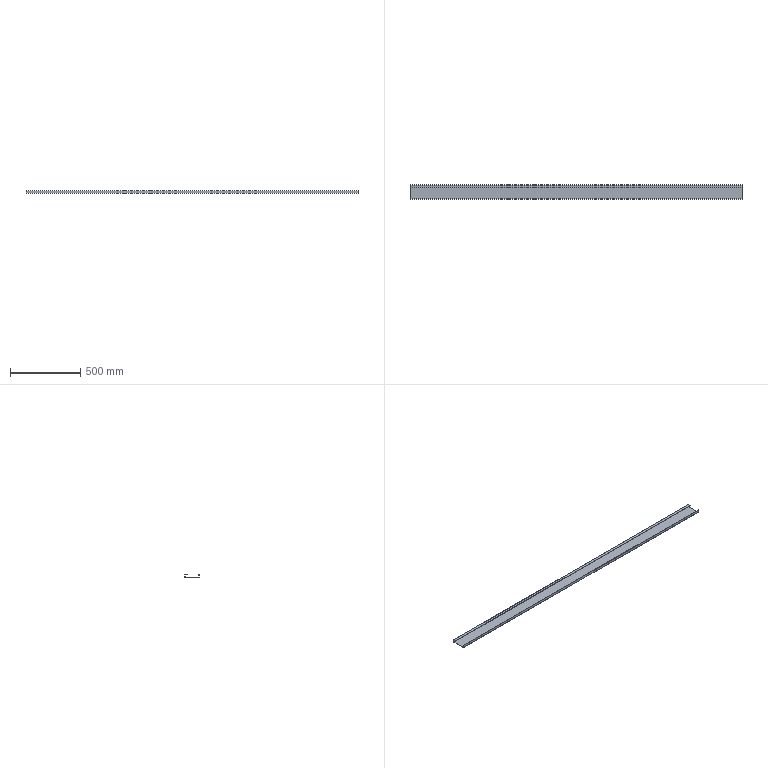Part | STEP file | 粉仓踢脚Plate 9 | 1 solid | 18 faces | box 2365 x 100 x 20 mm | volume 543643 mm3 | plane 12 | cylinder 6 | commonest cylinder face diameters 2 x3 5 x3
STEP:
#1=CARTESIAN_POINT('',(0.,0.,0.));
#2=DIRECTION('',(0.,0.,1.));
#3=DIRECTION('',(1.,0.,0.));
#4=AXIS2_PLACEMENT_3D('',#1,#2,#3);
#5=CARTESIAN_POINT('',(-1182.5,1.5,2.5));
#6=VERTEX_POINT('',#5);
#7=CARTESIAN_POINT('',(-1182.5,1.5,20.));
#8=VERTEX_POINT('',#7);
#9=CARTESIAN_POINT('',(-1182.5,1.5,2.5));
#10=DIRECTION('',(0.,0.,1.));
#11=VECTOR('',#10,1.);
#12=LINE('',#9,#11);
#13=CARTESIAN_POINT('',(1182.5,1.5,2.5));
#14=DIRECTION('',(0.,-1.,0.));
#15=DIRECTION('',(0.,0.,-1.));
#16=AXIS2_PLACEMENT_3D('',#13,#14,#15);
#17=PLANE('',#16);
#18=CARTESIAN_POINT('',(0.,-2365.));
#19=DIRECTION('',(-1.,0.));
#20=VECTOR('',#19,1.);
#21=LINE('',#18,#20);
#22=(GEOMETRIC_REPRESENTATION_CONTEXT(2)PARAMETRIC_REPRESENTATION_CONTEXT()REPRESENTATION_CONTEXT('',''));
#23=DEFINITIONAL_REPRESENTATION('',(#21),#22);
#24=PCURVE('',#17,#23);
#25=CARTESIAN_POINT('',(-1182.5,2.5,2.5));
#26=DIRECTION('',(-1.,0.,0.));
#27=DIRECTION('',(0.,0.,1.));
#28=AXIS2_PLACEMENT_3D('',#25,#26,#27);
#29=PLANE('',#28);
#30=CARTESIAN_POINT('',(0.,-1.));
#31=DIRECTION('',(1.,0.));
#32=VECTOR('',#31,1.);
#33=LINE('',#30,#32);
#34=(GEOMETRIC_REPRESENTATION_CONTEXT(2)PARAMETRIC_REPRESENTATION_CONTEXT()REPRESENTATION_CONTEXT('',''));
#35=DEFINITIONAL_REPRESENTATION('',(#33),#34);
#36=PCURVE('',#29,#35);
#37=SURFACE_CURVE('',#12,(#24,#36),.PCURVE_S1.);
#38=EDGE_CURVE('',#6,#8,#37,.T.);
#39=ORIENTED_EDGE('',*,*,#38,.T.);
#40=CARTESIAN_POINT('',(1182.5,1.5,20.));
#41=VERTEX_POINT('',#40);
#42=CARTESIAN_POINT('',(1182.5,1.5,20.));
#43=DIRECTION('',(-1.,0.,0.));
#44=VECTOR('',#43,1.);
#45=LINE('',#42,#44);
#46=CARTESIAN_POINT('',(-17.5,0.));
#47=DIRECTION('',(0.,-1.));
#48=VECTOR('',#47,1.);
#49=LINE('',#46,#48);
#50=(GEOMETRIC_REPRESENTATION_CONTEXT(2)PARAMETRIC_REPRESENTATION_CONTEXT()REPRESENTATION_CONTEXT('',''));
#51=DEFINITIONAL_REPRESENTATION('',(#49),#50);
#52=PCURVE('',#17,#51);
#53=CARTESIAN_POINT('',(1182.5,0.,20.));
#54=DIRECTION('',(0.,0.,1.));
#55=DIRECTION('',(1.,0.,0.));
#56=AXIS2_PLACEMENT_3D('',#53,#54,#55);
#57=PLANE('',#56);
#58=CARTESIAN_POINT('',(0.,1.5));
#59=DIRECTION('',(-1.,0.));
#60=VECTOR('',#59,1.);
#61=LINE('',#58,#60);
#62=(GEOMETRIC_REPRESENTATION_CONTEXT(2)PARAMETRIC_REPRESENTATION_CONTEXT()REPRESENTATION_CONTEXT('',''));
#63=DEFINITIONAL_REPRESENTATION('',(#61),#62);
#64=PCURVE('',#57,#63);
#65=SURFACE_CURVE('',#45,(#52,#64),.PCURVE_S1.);
#66=EDGE_CURVE('',#41,#8,#65,.T.);
#67=ORIENTED_EDGE('',*,*,#66,.F.);
#68=CARTESIAN_POINT('',(1182.5,1.5,2.5));
#69=VERTEX_POINT('',#68);
#70=CARTESIAN_POINT('',(1182.5,1.5,2.5));
#71=DIRECTION('',(0.,0.,1.));
#72=VECTOR('',#71,1.);
#73=LINE('',#70,#72);
#74=CARTESIAN_POINT('',(0.,0.));
#75=DIRECTION('',(-1.,0.));
#76=VECTOR('',#75,1.);
#77=LINE('',#74,#76);
#78=(GEOMETRIC_REPRESENTATION_CONTEXT(2)PARAMETRIC_REPRESENTATION_CONTEXT()REPRESENTATION_CONTEXT('',''));
#79=DEFINITIONAL_REPRESENTATION('',(#77),#78);
#80=PCURVE('',#17,#79);
#81=CARTESIAN_POINT('',(1182.5,2.5,2.5));
#82=DIRECTION('',(-1.,0.,0.));
#83=DIRECTION('',(0.,0.,1.));
#84=AXIS2_PLACEMENT_3D('',#81,#82,#83);
#85=PLANE('',#84);
#86=CARTESIAN_POINT('',(0.,-1.));
#87=DIRECTION('',(1.,0.));
#88=VECTOR('',#87,1.);
#89=LINE('',#86,#88);
#90=(GEOMETRIC_REPRESENTATION_CONTEXT(2)PARAMETRIC_REPRESENTATION_CONTEXT()REPRESENTATION_CONTEXT('',''));
#91=DEFINITIONAL_REPRESENTATION('',(#89),#90);
#92=PCURVE('',#85,#91);
#93=SURFACE_CURVE('',#73,(#80,#92),.PCURVE_S1.);
#94=EDGE_CURVE('',#69,#41,#93,.T.);
#95=ORIENTED_EDGE('',*,*,#94,.F.);
#96=CARTESIAN_POINT('',(1182.5,1.5,2.5));
#97=DIRECTION('',(-1.,0.,0.));
#98=VECTOR('',#97,1.);
#99=LINE('',#96,#98);
#100=CARTESIAN_POINT('',(0.,0.));
#101=DIRECTION('',(0.,-1.));
#102=VECTOR('',#101,1.);
#103=LINE('',#100,#102);
#104=(GEOMETRIC_REPRESENTATION_CONTEXT(2)PARAMETRIC_REPRESENTATION_CONTEXT()REPRESENTATION_CONTEXT('',''));
#105=DEFINITIONAL_REPRESENTATION('',(#103),#104);
#106=PCURVE('',#17,#105);
#107=CARTESIAN_POINT('',(1182.5,2.5,2.5));
#108=DIRECTION('',(-1.,0.,0.));
#109=DIRECTION('',(0.,0.,1.));
#110=AXIS2_PLACEMENT_3D('',#107,#108,#109);
#111=CYLINDRICAL_SURFACE('',#110,1.);
#112=CARTESIAN_POINT('',(4.712,0.));
#113=DIRECTION('',(0.,1.));
#114=VECTOR('',#113,1.);
#115=LINE('',#112,#114);
#116=(GEOMETRIC_REPRESENTATION_CONTEXT(2)PARAMETRIC_REPRESENTATION_CONTEXT()REPRESENTATION_CONTEXT('',''));
#117=DEFINITIONAL_REPRESENTATION('',(#115),#116);
#118=PCURVE('',#111,#117);
#119=SURFACE_CURVE('',#99,(#106,#118),.PCURVE_S1.);
#120=EDGE_CURVE('',#69,#6,#119,.T.);
#121=ORIENTED_EDGE('',*,*,#120,.T.);
#122=EDGE_LOOP('',(#39,#67,#95,#121));
#123=FACE_BOUND('',#122,.T.);
#124=ADVANCED_FACE('',(#123),#17,.F.);
#125=CARTESIAN_POINT('',(-1182.5,0.,20.));
#126=VERTEX_POINT('',#125);
#127=CARTESIAN_POINT('',(-1182.5,0.,20.));
#128=DIRECTION('',(0.,1.,0.));
#129=VECTOR('',#128,1.);
#130=LINE('',#127,#129);
#131=CARTESIAN_POINT('',(-2365.,0.));
#132=DIRECTION('',(0.,1.));
#133=VECTOR('',#132,1.);
#134=LINE('',#131,#133);
#135=(GEOMETRIC_REPRESENTATION_CONTEXT(2)PARAMETRIC_REPRESENTATION_CONTEXT()REPRESENTATION_CONTEXT('',''));
#136=DEFINITIONAL_REPRESENTATION('',(#134),#135);
#137=PCURVE('',#57,#136);
#138=CARTESIAN_POINT('',(17.5,-2.5));
#139=DIRECTION('',(0.,1.));
#140=VECTOR('',#139,1.);
#141=LINE('',#138,#140);
#142=(GEOMETRIC_REPRESENTATION_CONTEXT(2)PARAMETRIC_REPRESENTATION_CONTEXT()REPRESENTATION_CONTEXT('',''));
#143=DEFINITIONAL_REPRESENTATION('',(#141),#142);
#144=PCURVE('',#29,#143);
#145=SURFACE_CURVE('',#130,(#137,#144),.PCURVE_S1.);
#146=EDGE_CURVE('',#126,#8,#145,.T.);
#147=ORIENTED_EDGE('',*,*,#146,.F.);
#148=CARTESIAN_POINT('',(1182.5,0.,20.));
#149=VERTEX_POINT('',#148);
#150=CARTESIAN_POINT('',(1182.5,0.,20.));
#151=DIRECTION('',(-1.,0.,0.));
#152=VECTOR('',#151,1.);
#153=LINE('',#150,#152);
#154=CARTESIAN_POINT('',(0.,0.));
#155=DIRECTION('',(-1.,0.));
#156=VECTOR('',#155,1.);
#157=LINE('',#154,#156);
#158=(GEOMETRIC_REPRESENTATION_CONTEXT(2)PARAMETRIC_REPRESENTATION_CONTEXT()REPRESENTATION_CONTEXT('',''));
#159=DEFINITIONAL_REPRESENTATION('',(#157),#158);
#160=PCURVE('',#57,#159);
#161=CARTESIAN_POINT('',(1182.5,0.,2.5));
#162=DIRECTION('',(0.,-1.,0.));
#163=DIRECTION('',(0.,0.,-1.));
#164=AXIS2_PLACEMENT_3D('',#161,#162,#163);
#165=PLANE('',#164);
#166=CARTESIAN_POINT('',(-17.5,0.));
#167=DIRECTION('',(0.,-1.));
#168=VECTOR('',#167,1.);
#169=LINE('',#166,#168);
#170=(GEOMETRIC_REPRESENTATION_CONTEXT(2)PARAMETRIC_REPRESENTATION_CONTEXT()REPRESENTATION_CONTEXT('',''));
#171=DEFINITIONAL_REPRESENTATION('',(#169),#170);
#172=PCURVE('',#165,#171);
#173=SURFACE_CURVE('',#153,(#160,#172),.PCURVE_S1.);
#174=EDGE_CURVE('',#149,#126,#173,.T.);
#175=ORIENTED_EDGE('',*,*,#174,.F.);
#176=CARTESIAN_POINT('',(1182.5,0.,20.));
#177=DIRECTION('',(0.,1.,0.));
#178=VECTOR('',#177,1.);
#179=LINE('',#176,#178);
#180=CARTESIAN_POINT('',(0.,0.));
#181=DIRECTION('',(0.,1.));
#182=VECTOR('',#181,1.);
#183=LINE('',#180,#182);
#184=(GEOMETRIC_REPRESENTATION_CONTEXT(2)PARAMETRIC_REPRESENTATION_CONTEXT()REPRESENTATION_CONTEXT('',''));
#185=DEFINITIONAL_REPRESENTATION('',(#183),#184);
#186=PCURVE('',#57,#185);
#187=CARTESIAN_POINT('',(17.5,-2.5));
#188=DIRECTION('',(0.,1.));
#189=VECTOR('',#188,1.);
#190=LINE('',#187,#189);
#191=(GEOMETRIC_REPRESENTATION_CONTEXT(2)PARAMETRIC_REPRESENTATION_CONTEXT()REPRESENTATION_CONTEXT('',''));
#192=DEFINITIONAL_REPRESENTATION('',(#190),#191);
#193=PCURVE('',#85,#192);
#194=SURFACE_CURVE('',#179,(#186,#193),.PCURVE_S1.);
#195=EDGE_CURVE('',#149,#41,#194,.T.);
#196=ORIENTED_EDGE('',*,*,#195,.T.);
#197=ORIENTED_EDGE('',*,*,#66,.T.);
#198=EDGE_LOOP('',(#147,#175,#196,#197));
#199=FACE_BOUND('',#198,.T.);
#200=ADVANCED_FACE('',(#199),#57,.T.);
#201=CARTESIAN_POINT('',(-1182.5,0.,2.5));
#202=VERTEX_POINT('',#201);
#203=CARTESIAN_POINT('',(-1182.5,0.,2.5));
#204=DIRECTION('',(0.,0.,1.));
#205=VECTOR('',#204,1.);
#206=LINE('',#203,#205);
#207=CARTESIAN_POINT('',(0.,-2365.));
#208=DIRECTION('',(-1.,0.));
#209=VECTOR('',#208,1.);
#210=LINE('',#207,#209);
#211=(GEOMETRIC_REPRESENTATION_CONTEXT(2)PARAMETRIC_REPRESENTATION_CONTEXT()REPRESENTATION_CONTEXT('',''));
#212=DEFINITIONAL_REPRESENTATION('',(#210),#211);
#213=PCURVE('',#165,#212);
#214=CARTESIAN_POINT('',(0.,-2.5));
#215=DIRECTION('',(1.,0.));
#216=VECTOR('',#215,1.);
#217=LINE('',#214,#216);
#218=(GEOMETRIC_REPRESENTATION_CONTEXT(2)PARAMETRIC_REPRESENTATION_CONTEXT()REPRESENTATION_CONTEXT('',''));
#219=DEFINITIONAL_REPRESENTATION('',(#217),#218);
#220=PCURVE('',#29,#219);
#221=SURFACE_CURVE('',#206,(#213,#220),.PCURVE_S1.);
#222=EDGE_CURVE('',#202,#126,#221,.T.);
#223=ORIENTED_EDGE('',*,*,#222,.F.);
#224=CARTESIAN_POINT('',(1182.5,0.,2.5));
#225=VERTEX_POINT('',#224);
#226=CARTESIAN_POINT('',(1182.5,0.,2.5));
#227=DIRECTION('',(-1.,0.,0.));
#228=VECTOR('',#227,1.);
#229=LINE('',#226,#228);
#230=CARTESIAN_POINT('',(0.,0.));
#231=DIRECTION('',(0.,-1.));
#232=VECTOR('',#231,1.);
#233=LINE('',#230,#232);
#234=(GEOMETRIC_REPRESENTATION_CONTEXT(2)PARAMETRIC_REPRESENTATION_CONTEXT()REPRESENTATION_CONTEXT('',''));
#235=DEFINITIONAL_REPRESENTATION('',(#233),#234);
#236=PCURVE('',#165,#235);
#237=CARTESIAN_POINT('',(1182.5,2.5,2.5));
#238=DIRECTION('',(-1.,0.,0.));
#239=DIRECTION('',(0.,0.,1.));
#240=AXIS2_PLACEMENT_3D('',#237,#238,#239);
#241=CYLINDRICAL_SURFACE('',#240,2.5);
#242=CARTESIAN_POINT('',(4.712,0.));
#243=DIRECTION('',(0.,1.));
#244=VECTOR('',#243,1.);
#245=LINE('',#242,#244);
#246=(GEOMETRIC_REPRESENTATION_CONTEXT(2)PARAMETRIC_REPRESENTATION_CONTEXT()REPRESENTATION_CONTEXT('',''));
#247=DEFINITIONAL_REPRESENTATION('',(#245),#246);
#248=PCURVE('',#241,#247);
#249=SURFACE_CURVE('',#229,(#236,#248),.PCURVE_S1.);
#250=EDGE_CURVE('',#225,#202,#249,.T.);
#251=ORIENTED_EDGE('',*,*,#250,.F.);
#252=CARTESIAN_POINT('',(1182.5,0.,2.5));
#253=DIRECTION('',(0.,0.,1.));
#254=VECTOR('',#253,1.);
#255=LINE('',#252,#254);
#256=CARTESIAN_POINT('',(0.,0.));
#257=DIRECTION('',(-1.,0.));
#258=VECTOR('',#257,1.);
#259=LINE('',#256,#258);
#260=(GEOMETRIC_REPRESENTATION_CONTEXT(2)PARAMETRIC_REPRESENTATION_CONTEXT()REPRESENTATION_CONTEXT('',''));
#261=DEFINITIONAL_REPRESENTATION('',(#259),#260);
#262=PCURVE('',#165,#261);
#263=CARTESIAN_POINT('',(0.,-2.5));
#264=DIRECTION('',(1.,0.));
#265=VECTOR('',#264,1.);
#266=LINE('',#263,#265);
#267=(GEOMETRIC_REPRESENTATION_CONTEXT(2)PARAMETRIC_REPRESENTATION_CONTEXT()REPRESENTATION_CONTEXT('',''));
#268=DEFINITIONAL_REPRESENTATION('',(#266),#267);
#269=PCURVE('',#85,#268);
#270=SURFACE_CURVE('',#255,(#262,#269),.PCURVE_S1.);
#271=EDGE_CURVE('',#225,#149,#270,.T.);
#272=ORIENTED_EDGE('',*,*,#271,.T.);
#273=ORIENTED_EDGE('',*,*,#174,.T.);
#274=EDGE_LOOP('',(#223,#251,#272,#273));
#275=FACE_BOUND('',#274,.T.);
#276=ADVANCED_FACE('',(#275),#165,.T.);
#277=CARTESIAN_POINT('',(-1182.5,2.5,0.));
#278=VERTEX_POINT('',#277);
#279=CARTESIAN_POINT('',(-1182.5,2.5,2.5));
#280=DIRECTION('',(-1.,0.,0.));
#281=DIRECTION('',(0.,0.,1.));
#282=AXIS2_PLACEMENT_3D('',#279,#280,#281);
#283=CIRCLE('',#282,2.5);
#284=CARTESIAN_POINT('',(0.,2365.));
#285=DIRECTION('',(1.,0.));
#286=VECTOR('',#285,1.);
#287=LINE('',#284,#286);
#288=(GEOMETRIC_REPRESENTATION_CONTEXT(2)PARAMETRIC_REPRESENTATION_CONTEXT()REPRESENTATION_CONTEXT('',''));
#289=DEFINITIONAL_REPRESENTATION('',(#287),#288);
#290=PCURVE('',#241,#289);
#291=CARTESIAN_POINT('',(0.,0.));
#292=DIRECTION('',(1.,0.));
#293=AXIS2_PLACEMENT_2D('',#291,#292);
#294=CIRCLE('',#293,2.5);
#295=(GEOMETRIC_REPRESENTATION_CONTEXT(2)PARAMETRIC_REPRESENTATION_CONTEXT()REPRESENTATION_CONTEXT('',''));
#296=DEFINITIONAL_REPRESENTATION('',(#294),#295);
#297=PCURVE('',#29,#296);
#298=SURFACE_CURVE('',#283,(#290,#297),.PCURVE_S1.);
#299=EDGE_CURVE('',#278,#202,#298,.T.);
#300=ORIENTED_EDGE('',*,*,#299,.F.);
#301=CARTESIAN_POINT('',(1182.5,2.5,0.));
#302=VERTEX_POINT('',#301);
#303=CARTESIAN_POINT('',(1182.5,2.5,0.));
#304=DIRECTION('',(-1.,0.,0.));
#305=VECTOR('',#304,1.);
#306=LINE('',#303,#305);
#307=CARTESIAN_POINT('',(3.142,0.));
#308=DIRECTION('',(0.,1.));
#309=VECTOR('',#308,1.);
#310=LINE('',#307,#309);
#311=(GEOMETRIC_REPRESENTATION_CONTEXT(2)PARAMETRIC_REPRESENTATION_CONTEXT()REPRESENTATION_CONTEXT('',''));
#312=DEFINITIONAL_REPRESENTATION('',(#310),#311);
#313=PCURVE('',#241,#312);
#314=CARTESIAN_POINT('',(1182.5,2.5,0.));
#315=DIRECTION('',(0.,0.,-1.));
#316=DIRECTION('',(-1.,0.,0.));
#317=AXIS2_PLACEMENT_3D('',#314,#315,#316);
#318=PLANE('',#317);
#319=CARTESIAN_POINT('',(0.,0.));
#320=DIRECTION('',(1.,0.));
#321=VECTOR('',#320,1.);
#322=LINE('',#319,#321);
#323=(GEOMETRIC_REPRESENTATION_CONTEXT(2)PARAMETRIC_REPRESENTATION_CONTEXT()REPRESENTATION_CONTEXT('',''));
#324=DEFINITIONAL_REPRESENTATION('',(#322),#323);
#325=PCURVE('',#318,#324);
#326=SURFACE_CURVE('',#306,(#313,#325),.PCURVE_S1.);
#327=EDGE_CURVE('',#302,#278,#326,.T.);
#328=ORIENTED_EDGE('',*,*,#327,.F.);
#329=CARTESIAN_POINT('',(1182.5,2.5,2.5));
#330=DIRECTION('',(-1.,0.,0.));
#331=DIRECTION('',(0.,0.,1.));
#332=AXIS2_PLACEMENT_3D('',#329,#330,#331);
#333=CIRCLE('',#332,2.5);
#334=CARTESIAN_POINT('',(0.,0.));
#335=DIRECTION('',(1.,0.));
#336=VECTOR('',#335,1.);
#337=LINE('',#334,#336);
#338=(GEOMETRIC_REPRESENTATION_CONTEXT(2)PARAMETRIC_REPRESENTATION_CONTEXT()REPRESENTATION_CONTEXT('',''));
#339=DEFINITIONAL_REPRESENTATION('',(#337),#338);
#340=PCURVE('',#241,#339);
#341=CARTESIAN_POINT('',(0.,0.));
#342=DIRECTION('',(1.,0.));
#343=AXIS2_PLACEMENT_2D('',#341,#342);
#344=CIRCLE('',#343,2.5);
#345=(GEOMETRIC_REPRESENTATION_CONTEXT(2)PARAMETRIC_REPRESENTATION_CONTEXT()REPRESENTATION_CONTEXT('',''));
#346=DEFINITIONAL_REPRESENTATION('',(#344),#345);
#347=PCURVE('',#85,#346);
#348=SURFACE_CURVE('',#333,(#340,#347),.PCURVE_S1.);
#349=EDGE_CURVE('',#302,#225,#348,.T.);
#350=ORIENTED_EDGE('',*,*,#349,.T.);
#351=ORIENTED_EDGE('',*,*,#250,.T.);
#352=EDGE_LOOP('',(#300,#328,#350,#351));
#353=FACE_BOUND('',#352,.T.);
#354=ADVANCED_FACE('',(#353),#241,.T.);
#355=CARTESIAN_POINT('',(-1182.5,97.5,0.));
#356=VERTEX_POINT('',#355);
#357=CARTESIAN_POINT('',(-1182.5,2.5,0.));
#358=DIRECTION('',(0.,-1.,0.));
#359=VECTOR('',#358,1.);
#360=LINE('',#357,#359);
#361=CARTESIAN_POINT('',(2365.,0.));
#362=DIRECTION('',(0.,-1.));
#363=VECTOR('',#362,1.);
#364=LINE('',#361,#363);
#365=(GEOMETRIC_REPRESENTATION_CONTEXT(2)PARAMETRIC_REPRESENTATION_CONTEXT()REPRESENTATION_CONTEXT('',''));
#366=DEFINITIONAL_REPRESENTATION('',(#364),#365);
#367=PCURVE('',#318,#366);
#368=CARTESIAN_POINT('',(-2.5,0.));
#369=DIRECTION('',(0.,-1.));
#370=VECTOR('',#369,1.);
#371=LINE('',#368,#370);
#372=(GEOMETRIC_REPRESENTATION_CONTEXT(2)PARAMETRIC_REPRESENTATION_CONTEXT()REPRESENTATION_CONTEXT('',''));
#373=DEFINITIONAL_REPRESENTATION('',(#371),#372);
#374=PCURVE('',#29,#373);
#375=SURFACE_CURVE('',#360,(#367,#374),.PCURVE_S1.);
#376=EDGE_CURVE('',#356,#278,#375,.T.);
#377=ORIENTED_EDGE('',*,*,#376,.F.);
#378=CARTESIAN_POINT('',(1182.5,97.5,0.));
#379=VERTEX_POINT('',#378);
#380=CARTESIAN_POINT('',(1182.5,97.5,0.));
#381=DIRECTION('',(-1.,0.,0.));
#382=VECTOR('',#381,1.);
#383=LINE('',#380,#382);
#384=CARTESIAN_POINT('',(0.,95.));
#385=DIRECTION('',(1.,0.));
#386=VECTOR('',#385,1.);
#387=LINE('',#384,#386);
#388=(GEOMETRIC_REPRESENTATION_CONTEXT(2)PARAMETRIC_REPRESENTATION_CONTEXT()REPRESENTATION_CONTEXT('',''));
#389=DEFINITIONAL_REPRESENTATION('',(#387),#388);
#390=PCURVE('',#318,#389);
#391=CARTESIAN_POINT('',(1182.5,97.5,2.5));
#392=DIRECTION('',(-1.,0.,0.));
#393=DIRECTION('',(0.,0.,1.));
#394=AXIS2_PLACEMENT_3D('',#391,#392,#393);
#395=CYLINDRICAL_SURFACE('',#394,2.5);
#396=CARTESIAN_POINT('',(3.142,0.));
#397=DIRECTION('',(0.,1.));
#398=VECTOR('',#397,1.);
#399=LINE('',#396,#398);
#400=(GEOMETRIC_REPRESENTATION_CONTEXT(2)PARAMETRIC_REPRESENTATION_CONTEXT()REPRESENTATION_CONTEXT('',''));
#401=DEFINITIONAL_REPRESENTATION('',(#399),#400);
#402=PCURVE('',#395,#401);
#403=SURFACE_CURVE('',#383,(#390,#402),.PCURVE_S1.);
#404=EDGE_CURVE('',#379,#356,#403,.T.);
#405=ORIENTED_EDGE('',*,*,#404,.F.);
#406=CARTESIAN_POINT('',(1182.5,2.5,0.));
#407=DIRECTION('',(0.,-1.,0.));
#408=VECTOR('',#407,1.);
#409=LINE('',#406,#408);
#410=CARTESIAN_POINT('',(0.,0.));
#411=DIRECTION('',(0.,-1.));
#412=VECTOR('',#411,1.);
#413=LINE('',#410,#412);
#414=(GEOMETRIC_REPRESENTATION_CONTEXT(2)PARAMETRIC_REPRESENTATION_CONTEXT()REPRESENTATION_CONTEXT('',''));
#415=DEFINITIONAL_REPRESENTATION('',(#413),#414);
#416=PCURVE('',#318,#415);
#417=CARTESIAN_POINT('',(-2.5,0.));
#418=DIRECTION('',(0.,-1.));
#419=VECTOR('',#418,1.);
#420=LINE('',#417,#419);
#421=(GEOMETRIC_REPRESENTATION_CONTEXT(2)PARAMETRIC_REPRESENTATION_CONTEXT()REPRESENTATION_CONTEXT('',''));
#422=DEFINITIONAL_REPRESENTATION('',(#420),#421);
#423=PCURVE('',#85,#422);
#424=SURFACE_CURVE('',#409,(#416,#423),.PCURVE_S1.);
#425=EDGE_CURVE('',#379,#302,#424,.T.);
#426=ORIENTED_EDGE('',*,*,#425,.T.);
#427=ORIENTED_EDGE('',*,*,#327,.T.);
#428=EDGE_LOOP('',(#377,#405,#426,#427));
#429=FACE_BOUND('',#428,.T.);
#430=ADVANCED_FACE('',(#429),#318,.T.);
#431=CARTESIAN_POINT('',(-1182.5,100.,2.5));
#432=VERTEX_POINT('',#431);
#433=CARTESIAN_POINT('',(-1182.5,97.5,2.5));
#434=DIRECTION('',(-1.,0.,0.));
#435=DIRECTION('',(0.,0.,-1.));
#436=AXIS2_PLACEMENT_3D('',#433,#434,#435);
#437=CIRCLE('',#436,2.5);
#438=CARTESIAN_POINT('',(-3.142,2365.));
#439=DIRECTION('',(1.,0.));
#440=VECTOR('',#439,1.);
#441=LINE('',#438,#440);
#442=(GEOMETRIC_REPRESENTATION_CONTEXT(2)PARAMETRIC_REPRESENTATION_CONTEXT()REPRESENTATION_CONTEXT('',''));
#443=DEFINITIONAL_REPRESENTATION('',(#441),#442);
#444=PCURVE('',#395,#443);
#445=CARTESIAN_POINT('',(0.,95.));
#446=DIRECTION('',(-1.,0.));
#447=AXIS2_PLACEMENT_2D('',#445,#446);
#448=CIRCLE('',#447,2.5);
#449=(GEOMETRIC_REPRESENTATION_CONTEXT(2)PARAMETRIC_REPRESENTATION_CONTEXT()REPRESENTATION_CONTEXT('',''));
#450=DEFINITIONAL_REPRESENTATION('',(#448),#449);
#451=PCURVE('',#29,#450);
#452=SURFACE_CURVE('',#437,(#444,#451),.PCURVE_S1.);
#453=EDGE_CURVE('',#432,#356,#452,.T.);
#454=ORIENTED_EDGE('',*,*,#453,.F.);
#455=CARTESIAN_POINT('',(1182.5,100.,2.5));
#456=VERTEX_POINT('',#455);
#457=CARTESIAN_POINT('',(1182.5,100.,2.5));
#458=DIRECTION('',(-1.,0.,0.));
#459=VECTOR('',#458,1.);
#460=LINE('',#457,#459);
#461=CARTESIAN_POINT('',(1.571,0.));
#462=DIRECTION('',(0.,1.));
#463=VECTOR('',#462,1.);
#464=LINE('',#461,#463);
#465=(GEOMETRIC_REPRESENTATION_CONTEXT(2)PARAMETRIC_REPRESENTATION_CONTEXT()REPRESENTATION_CONTEXT('',''));
#466=DEFINITIONAL_REPRESENTATION('',(#464),#465);
#467=PCURVE('',#395,#466);
#468=CARTESIAN_POINT('',(1182.5,100.,2.5));
#469=DIRECTION('',(0.,1.,0.));
#470=DIRECTION('',(0.,0.,1.));
#471=AXIS2_PLACEMENT_3D('',#468,#469,#470);
#472=PLANE('',#471);
#473=CARTESIAN_POINT('',(0.,0.));
#474=DIRECTION('',(0.,-1.));
#475=VECTOR('',#474,1.);
#476=LINE('',#473,#475);
#477=(GEOMETRIC_REPRESENTATION_CONTEXT(2)PARAMETRIC_REPRESENTATION_CONTEXT()REPRESENTATION_CONTEXT('',''));
#478=DEFINITIONAL_REPRESENTATION('',(#476),#477);
#479=PCURVE('',#472,#478);
#480=SURFACE_CURVE('',#460,(#467,#479),.PCURVE_S1.);
#481=EDGE_CURVE('',#456,#432,#480,.T.);
#482=ORIENTED_EDGE('',*,*,#481,.F.);
#483=CARTESIAN_POINT('',(1182.5,97.5,2.5));
#484=DIRECTION('',(-1.,0.,0.));
#485=DIRECTION('',(0.,0.,-1.));
#486=AXIS2_PLACEMENT_3D('',#483,#484,#485);
#487=CIRCLE('',#486,2.5);
#488=CARTESIAN_POINT('',(-3.142,0.));
#489=DIRECTION('',(1.,0.));
#490=VECTOR('',#489,1.);
#491=LINE('',#488,#490);
#492=(GEOMETRIC_REPRESENTATION_CONTEXT(2)PARAMETRIC_REPRESENTATION_CONTEXT()REPRESENTATION_CONTEXT('',''));
#493=DEFINITIONAL_REPRESENTATION('',(#491),#492);
#494=PCURVE('',#395,#493);
#495=CARTESIAN_POINT('',(0.,95.));
#496=DIRECTION('',(-1.,0.));
#497=AXIS2_PLACEMENT_2D('',#495,#496);
#498=CIRCLE('',#497,2.5);
#499=(GEOMETRIC_REPRESENTATION_CONTEXT(2)PARAMETRIC_REPRESENTATION_CONTEXT()REPRESENTATION_CONTEXT('',''));
#500=DEFINITIONAL_REPRESENTATION('',(#498),#499);
#501=PCURVE('',#85,#500);
#502=SURFACE_CURVE('',#487,(#494,#501),.PCURVE_S1.);
#503=EDGE_CURVE('',#456,#379,#502,.T.);
#504=ORIENTED_EDGE('',*,*,#503,.T.);
#505=ORIENTED_EDGE('',*,*,#404,.T.);
#506=EDGE_LOOP('',(#454,#482,#504,#505));
#507=FACE_BOUND('',#506,.T.);
#508=ADVANCED_FACE('',(#507),#395,.T.);
#509=CARTESIAN_POINT('',(-1182.5,100.,17.5));
#510=VERTEX_POINT('',#509);
#511=CARTESIAN_POINT('',(-1182.5,100.,2.5));
#512=DIRECTION('',(0.,0.,-1.));
#513=VECTOR('',#512,1.);
#514=LINE('',#511,#513);
#515=CARTESIAN_POINT('',(0.,-2365.));
#516=DIRECTION('',(-1.,0.));
#517=VECTOR('',#516,1.);
#518=LINE('',#515,#517);
#519=(GEOMETRIC_REPRESENTATION_CONTEXT(2)PARAMETRIC_REPRESENTATION_CONTEXT()REPRESENTATION_CONTEXT('',''));
#520=DEFINITIONAL_REPRESENTATION('',(#518),#519);
#521=PCURVE('',#472,#520);
#522=CARTESIAN_POINT('',(0.,97.5));
#523=DIRECTION('',(-1.,0.));
#524=VECTOR('',#523,1.);
#525=LINE('',#522,#524);
#526=(GEOMETRIC_REPRESENTATION_CONTEXT(2)PARAMETRIC_REPRESENTATION_CONTEXT()REPRESENTATION_CONTEXT('',''));
#527=DEFINITIONAL_REPRESENTATION('',(#525),#526);
#528=PCURVE('',#29,#527);
#529=SURFACE_CURVE('',#514,(#521,#528),.PCURVE_S1.);
#530=EDGE_CURVE('',#510,#432,#529,.T.);
#531=ORIENTED_EDGE('',*,*,#530,.F.);
#532=CARTESIAN_POINT('',(1182.5,100.,17.5));
#533=VERTEX_POINT('',#532);
#534=CARTESIAN_POINT('',(1182.5,100.,17.5));
#535=DIRECTION('',(-1.,0.,0.));
#536=VECTOR('',#535,1.);
#537=LINE('',#534,#536);
#538=CARTESIAN_POINT('',(15.,0.));
#539=DIRECTION('',(0.,-1.));
#540=VECTOR('',#539,1.);
#541=LINE('',#538,#540);
#542=(GEOMETRIC_REPRESENTATION_CONTEXT(2)PARAMETRIC_REPRESENTATION_CONTEXT()REPRESENTATION_CONTEXT('',''));
#543=DEFINITIONAL_REPRESENTATION('',(#541),#542);
#544=PCURVE('',#472,#543);
#545=CARTESIAN_POINT('',(1182.5,97.5,17.5));
#546=DIRECTION('',(-1.,0.,0.));
#547=DIRECTION('',(0.,0.,1.));
#548=AXIS2_PLACEMENT_3D('',#545,#546,#547);
#549=CYLINDRICAL_SURFACE('',#548,2.5);
#550=CARTESIAN_POINT('',(1.571,0.));
#551=DIRECTION('',(0.,1.));
#552=VECTOR('',#551,1.);
#553=LINE('',#550,#552);
#554=(GEOMETRIC_REPRESENTATION_CONTEXT(2)PARAMETRIC_REPRESENTATION_CONTEXT()REPRESENTATION_CONTEXT('',''));
#555=DEFINITIONAL_REPRESENTATION('',(#553),#554);
#556=PCURVE('',#549,#555);
#557=SURFACE_CURVE('',#537,(#544,#556),.PCURVE_S1.);
#558=EDGE_CURVE('',#533,#510,#557,.T.);
#559=ORIENTED_EDGE('',*,*,#558,.F.);
#560=CARTESIAN_POINT('',(1182.5,100.,2.5));
#561=DIRECTION('',(0.,0.,-1.));
#562=VECTOR('',#561,1.);
#563=LINE('',#560,#562);
#564=CARTESIAN_POINT('',(0.,0.));
#565=DIRECTION('',(-1.,0.));
#566=VECTOR('',#565,1.);
#567=LINE('',#564,#566);
#568=(GEOMETRIC_REPRESENTATION_CONTEXT(2)PARAMETRIC_REPRESENTATION_CONTEXT()REPRESENTATION_CONTEXT('',''));
#569=DEFINITIONAL_REPRESENTATION('',(#567),#568);
#570=PCURVE('',#472,#569);
#571=CARTESIAN_POINT('',(0.,97.5));
#572=DIRECTION('',(-1.,0.));
#573=VECTOR('',#572,1.);
#574=LINE('',#571,#573);
#575=(GEOMETRIC_REPRESENTATION_CONTEXT(2)PARAMETRIC_REPRESENTATION_CONTEXT()REPRESENTATION_CONTEXT('',''));
#576=DEFINITIONAL_REPRESENTATION('',(#574),#575);
#577=PCURVE('',#85,#576);
#578=SURFACE_CURVE('',#563,(#570,#577),.PCURVE_S1.);
#579=EDGE_CURVE('',#533,#456,#578,.T.);
#580=ORIENTED_EDGE('',*,*,#579,.T.);
#581=ORIENTED_EDGE('',*,*,#481,.T.);
#582=EDGE_LOOP('',(#531,#559,#580,#581));
#583=FACE_BOUND('',#582,.T.);
#584=ADVANCED_FACE('',(#583),#472,.T.);
#585=CARTESIAN_POINT('',(-1182.5,97.5,20.));
#586=VERTEX_POINT('',#585);
#587=CARTESIAN_POINT('',(-1182.5,97.5,17.5));
#588=DIRECTION('',(-1.,0.,0.));
#589=DIRECTION('',(0.,0.,-1.));
#590=AXIS2_PLACEMENT_3D('',#587,#588,#589);
#591=CIRCLE('',#590,2.5);
#592=CARTESIAN_POINT('',(-3.142,2365.));
#593=DIRECTION('',(1.,0.));
#594=VECTOR('',#593,1.);
#595=LINE('',#592,#594);
#596=(GEOMETRIC_REPRESENTATION_CONTEXT(2)PARAMETRIC_REPRESENTATION_CONTEXT()REPRESENTATION_CONTEXT('',''));
#597=DEFINITIONAL_REPRESENTATION('',(#595),#596);
#598=PCURVE('',#549,#597);
#599=CARTESIAN_POINT('',(15.,95.));
#600=DIRECTION('',(-1.,0.));
#601=AXIS2_PLACEMENT_2D('',#599,#600);
#602=CIRCLE('',#601,2.5);
#603=(GEOMETRIC_REPRESENTATION_CONTEXT(2)PARAMETRIC_REPRESENTATION_CONTEXT()REPRESENTATION_CONTEXT('',''));
#604=DEFINITIONAL_REPRESENTATION('',(#602),#603);
#605=PCURVE('',#29,#604);
#606=SURFACE_CURVE('',#591,(#598,#605),.PCURVE_S1.);
#607=EDGE_CURVE('',#586,#510,#606,.T.);
#608=ORIENTED_EDGE('',*,*,#607,.F.);
#609=CARTESIAN_POINT('',(1182.5,97.5,20.));
#610=VERTEX_POINT('',#609);
#611=CARTESIAN_POINT('',(1182.5,97.5,20.));
#612=DIRECTION('',(-1.,0.,0.));
#613=VECTOR('',#612,1.);
#614=LINE('',#611,#613);
#615=CARTESIAN_POINT('',(0.,0.));
#616=DIRECTION('',(0.,1.));
#617=VECTOR('',#616,1.);
#618=LINE('',#615,#617);
#619=(GEOMETRIC_REPRESENTATION_CONTEXT(2)PARAMETRIC_REPRESENTATION_CONTEXT()REPRESENTATION_CONTEXT('',''));
#620=DEFINITIONAL_REPRESENTATION('',(#618),#619);
#621=PCURVE('',#549,#620);
#622=CARTESIAN_POINT('',(1182.5,97.5,20.));
#623=DIRECTION('',(0.,0.,1.));
#624=DIRECTION('',(1.,0.,0.));
#625=AXIS2_PLACEMENT_3D('',#622,#623,#624);
#626=PLANE('',#625);
#627=CARTESIAN_POINT('',(0.,0.));
#628=DIRECTION('',(-1.,0.));
#629=VECTOR('',#628,1.);
#630=LINE('',#627,#629);
#631=(GEOMETRIC_REPRESENTATION_CONTEXT(2)PARAMETRIC_REPRESENTATION_CONTEXT()REPRESENTATION_CONTEXT('',''));
#632=DEFINITIONAL_REPRESENTATION('',(#630),#631);
#633=PCURVE('',#626,#632);
#634=SURFACE_CURVE('',#614,(#621,#633),.PCURVE_S1.);
#635=EDGE_CURVE('',#610,#586,#634,.T.);
#636=ORIENTED_EDGE('',*,*,#635,.F.);
#637=CARTESIAN_POINT('',(1182.5,97.5,17.5));
#638=DIRECTION('',(-1.,0.,0.));
#639=DIRECTION('',(0.,0.,-1.));
#640=AXIS2_PLACEMENT_3D('',#637,#638,#639);
#641=CIRCLE('',#640,2.5);
#642=CARTESIAN_POINT('',(-3.142,0.));
#643=DIRECTION('',(1.,0.));
#644=VECTOR('',#643,1.);
#645=LINE('',#642,#644);
#646=(GEOMETRIC_REPRESENTATION_CONTEXT(2)PARAMETRIC_REPRESENTATION_CONTEXT()REPRESENTATION_CONTEXT('',''));
#647=DEFINITIONAL_REPRESENTATION('',(#645),#646);
#648=PCURVE('',#549,#647);
#649=CARTESIAN_POINT('',(15.,95.));
#650=DIRECTION('',(-1.,0.));
#651=AXIS2_PLACEMENT_2D('',#649,#650);
#652=CIRCLE('',#651,2.5);
#653=(GEOMETRIC_REPRESENTATION_CONTEXT(2)PARAMETRIC_REPRESENTATION_CONTEXT()REPRESENTATION_CONTEXT('',''));
#654=DEFINITIONAL_REPRESENTATION('',(#652),#653);
#655=PCURVE('',#85,#654);
#656=SURFACE_CURVE('',#641,(#648,#655),.PCURVE_S1.);
#657=EDGE_CURVE('',#610,#533,#656,.T.);
#658=ORIENTED_EDGE('',*,*,#657,.T.);
#659=ORIENTED_EDGE('',*,*,#558,.T.);
#660=EDGE_LOOP('',(#608,#636,#658,#659));
#661=FACE_BOUND('',#660,.T.);
#662=ADVANCED_FACE('',(#661),#549,.T.);
#663=CARTESIAN_POINT('',(-1182.5,80.,20.));
#664=VERTEX_POINT('',#663);
#665=CARTESIAN_POINT('',(-1182.5,97.5,20.));
#666=DIRECTION('',(0.,1.,0.));
#667=VECTOR('',#666,1.);
#668=LINE('',#665,#667);
#669=CARTESIAN_POINT('',(-2365.,0.));
#670=DIRECTION('',(0.,1.));
#671=VECTOR('',#670,1.);
#672=LINE('',#669,#671);
#673=(GEOMETRIC_REPRESENTATION_CONTEXT(2)PARAMETRIC_REPRESENTATION_CONTEXT()REPRESENTATION_CONTEXT('',''));
#674=DEFINITIONAL_REPRESENTATION('',(#672),#673);
#675=PCURVE('',#626,#674);
#676=CARTESIAN_POINT('',(17.5,95.));
#677=DIRECTION('',(0.,1.));
#678=VECTOR('',#677,1.);
#679=LINE('',#676,#678);
#680=(GEOMETRIC_REPRESENTATION_CONTEXT(2)PARAMETRIC_REPRESENTATION_CONTEXT()REPRESENTATION_CONTEXT('',''));
#681=DEFINITIONAL_REPRESENTATION('',(#679),#680);
#682=PCURVE('',#29,#681);
#683=SURFACE_CURVE('',#668,(#675,#682),.PCURVE_S1.);
#684=EDGE_CURVE('',#664,#586,#683,.T.);
#685=ORIENTED_EDGE('',*,*,#684,.F.);
#686=CARTESIAN_POINT('',(1182.5,80.,20.));
#687=VERTEX_POINT('',#686);
#688=CARTESIAN_POINT('',(1182.5,80.,20.));
#689=DIRECTION('',(-1.,0.,0.));
#690=VECTOR('',#689,1.);
#691=LINE('',#688,#690);
#692=CARTESIAN_POINT('',(0.,-17.5));
#693=DIRECTION('',(-1.,0.));
#694=VECTOR('',#693,1.);
#695=LINE('',#692,#694);
#696=(GEOMETRIC_REPRESENTATION_CONTEXT(2)PARAMETRIC_REPRESENTATION_CONTEXT()REPRESENTATION_CONTEXT('',''));
#697=DEFINITIONAL_REPRESENTATION('',(#695),#696);
#698=PCURVE('',#626,#697);
#699=CARTESIAN_POINT('',(1182.5,80.,18.5));
#700=DIRECTION('',(0.,-1.,0.));
#701=DIRECTION('',(0.,0.,-1.));
#702=AXIS2_PLACEMENT_3D('',#699,#700,#701);
#703=PLANE('',#702);
#704=CARTESIAN_POINT('',(-1.5,0.));
#705=DIRECTION('',(0.,-1.));
#706=VECTOR('',#705,1.);
#707=LINE('',#704,#706);
#708=(GEOMETRIC_REPRESENTATION_CONTEXT(2)PARAMETRIC_REPRESENTATION_CONTEXT()REPRESENTATION_CONTEXT('',''));
#709=DEFINITIONAL_REPRESENTATION('',(#707),#708);
#710=PCURVE('',#703,#709);
#711=SURFACE_CURVE('',#691,(#698,#710),.PCURVE_S1.);
#712=EDGE_CURVE('',#687,#664,#711,.T.);
#713=ORIENTED_EDGE('',*,*,#712,.F.);
#714=CARTESIAN_POINT('',(1182.5,97.5,20.));
#715=DIRECTION('',(0.,1.,0.));
#716=VECTOR('',#715,1.);
#717=LINE('',#714,#716);
#718=CARTESIAN_POINT('',(0.,0.));
#719=DIRECTION('',(0.,1.));
#720=VECTOR('',#719,1.);
#721=LINE('',#718,#720);
#722=(GEOMETRIC_REPRESENTATION_CONTEXT(2)PARAMETRIC_REPRESENTATION_CONTEXT()REPRESENTATION_CONTEXT('',''));
#723=DEFINITIONAL_REPRESENTATION('',(#721),#722);
#724=PCURVE('',#626,#723);
#725=CARTESIAN_POINT('',(17.5,95.));
#726=DIRECTION('',(0.,1.));
#727=VECTOR('',#726,1.);
#728=LINE('',#725,#727);
#729=(GEOMETRIC_REPRESENTATION_CONTEXT(2)PARAMETRIC_REPRESENTATION_CONTEXT()REPRESENTATION_CONTEXT('',''));
#730=DEFINITIONAL_REPRESENTATION('',(#728),#729);
#731=PCURVE('',#85,#730);
#732=SURFACE_CURVE('',#717,(#724,#731),.PCURVE_S1.);
#733=EDGE_CURVE('',#687,#610,#732,.T.);
#734=ORIENTED_EDGE('',*,*,#733,.T.);
#735=ORIENTED_EDGE('',*,*,#635,.T.);
#736=EDGE_LOOP('',(#685,#713,#734,#735));
#737=FACE_BOUND('',#736,.T.);
#738=ADVANCED_FACE('',(#737),#626,.T.);
#739=CARTESIAN_POINT('',(-1182.5,80.,18.5));
#740=VERTEX_POINT('',#739);
#741=CARTESIAN_POINT('',(-1182.5,80.,18.5));
#742=DIRECTION('',(0.,0.,1.));
#743=VECTOR('',#742,1.);
#744=LINE('',#741,#743);
#745=CARTESIAN_POINT('',(0.,-2365.));
#746=DIRECTION('',(-1.,0.));
#747=VECTOR('',#746,1.);
#748=LINE('',#745,#747);
#749=(GEOMETRIC_REPRESENTATION_CONTEXT(2)PARAMETRIC_REPRESENTATION_CONTEXT()REPRESENTATION_CONTEXT('',''));
#750=DEFINITIONAL_REPRESENTATION('',(#748),#749);
#751=PCURVE('',#703,#750);
#752=CARTESIAN_POINT('',(16.,77.5));
#753=DIRECTION('',(1.,0.));
#754=VECTOR('',#753,1.);
#755=LINE('',#752,#754);
#756=(GEOMETRIC_REPRESENTATION_CONTEXT(2)PARAMETRIC_REPRESENTATION_CONTEXT()REPRESENTATION_CONTEXT('',''));
#757=DEFINITIONAL_REPRESENTATION('',(#755),#756);
#758=PCURVE('',#29,#757);
#759=SURFACE_CURVE('',#744,(#751,#758),.PCURVE_S1.);
#760=EDGE_CURVE('',#740,#664,#759,.T.);
#761=ORIENTED_EDGE('',*,*,#760,.F.);
#762=CARTESIAN_POINT('',(1182.5,80.,18.5));
#763=VERTEX_POINT('',#762);
#764=CARTESIAN_POINT('',(1182.5,80.,18.5));
#765=DIRECTION('',(-1.,0.,0.));
#766=VECTOR('',#765,1.);
#767=LINE('',#764,#766);
#768=CARTESIAN_POINT('',(0.,0.));
#769=DIRECTION('',(0.,-1.));
#770=VECTOR('',#769,1.);
#771=LINE('',#768,#770);
#772=(GEOMETRIC_REPRESENTATION_CONTEXT(2)PARAMETRIC_REPRESENTATION_CONTEXT()REPRESENTATION_CONTEXT('',''));
#773=DEFINITIONAL_REPRESENTATION('',(#771),#772);
#774=PCURVE('',#703,#773);
#775=CARTESIAN_POINT('',(1182.5,97.5,18.5));
#776=DIRECTION('',(0.,0.,1.));
#777=DIRECTION('',(1.,0.,0.));
#778=AXIS2_PLACEMENT_3D('',#775,#776,#777);
#779=PLANE('',#778);
#780=CARTESIAN_POINT('',(0.,-17.5));
#781=DIRECTION('',(-1.,0.));
#782=VECTOR('',#781,1.);
#783=LINE('',#780,#782);
#784=(GEOMETRIC_REPRESENTATION_CONTEXT(2)PARAMETRIC_REPRESENTATION_CONTEXT()REPRESENTATION_CONTEXT('',''));
#785=DEFINITIONAL_REPRESENTATION('',(#783),#784);
#786=PCURVE('',#779,#785);
#787=SURFACE_CURVE('',#767,(#774,#786),.PCURVE_S1.);
#788=EDGE_CURVE('',#763,#740,#787,.T.);
#789=ORIENTED_EDGE('',*,*,#788,.F.);
#790=CARTESIAN_POINT('',(1182.5,80.,18.5));
#791=DIRECTION('',(0.,0.,1.));
#792=VECTOR('',#791,1.);
#793=LINE('',#790,#792);
#794=CARTESIAN_POINT('',(0.,0.));
#795=DIRECTION('',(-1.,0.));
#796=VECTOR('',#795,1.);
#797=LINE('',#794,#796);
#798=(GEOMETRIC_REPRESENTATION_CONTEXT(2)PARAMETRIC_REPRESENTATION_CONTEXT()REPRESENTATION_CONTEXT('',''));
#799=DEFINITIONAL_REPRESENTATION('',(#797),#798);
#800=PCURVE('',#703,#799);
#801=CARTESIAN_POINT('',(16.,77.5));
#802=DIRECTION('',(1.,0.));
#803=VECTOR('',#802,1.);
#804=LINE('',#801,#803);
#805=(GEOMETRIC_REPRESENTATION_CONTEXT(2)PARAMETRIC_REPRESENTATION_CONTEXT()REPRESENTATION_CONTEXT('',''));
#806=DEFINITIONAL_REPRESENTATION('',(#804),#805);
#807=PCURVE('',#85,#806);
#808=SURFACE_CURVE('',#793,(#800,#807),.PCURVE_S1.);
#809=EDGE_CURVE('',#763,#687,#808,.T.);
#810=ORIENTED_EDGE('',*,*,#809,.T.);
#811=ORIENTED_EDGE('',*,*,#712,.T.);
#812=EDGE_LOOP('',(#761,#789,#810,#811));
#813=FACE_BOUND('',#812,.T.);
#814=ADVANCED_FACE('',(#813),#703,.T.);
#815=CARTESIAN_POINT('',(-1182.5,97.5,18.5));
#816=VERTEX_POINT('',#815);
#817=CARTESIAN_POINT('',(-1182.5,97.5,18.5));
#818=DIRECTION('',(0.,1.,0.));
#819=VECTOR('',#818,1.);
#820=LINE('',#817,#819);
#821=CARTESIAN_POINT('',(-2365.,0.));
#822=DIRECTION('',(0.,1.));
#823=VECTOR('',#822,1.);
#824=LINE('',#821,#823);
#825=(GEOMETRIC_REPRESENTATION_CONTEXT(2)PARAMETRIC_REPRESENTATION_CONTEXT()REPRESENTATION_CONTEXT('',''));
#826=DEFINITIONAL_REPRESENTATION('',(#824),#825);
#827=PCURVE('',#779,#826);
#828=CARTESIAN_POINT('',(16.,95.));
#829=DIRECTION('',(0.,1.));
#830=VECTOR('',#829,1.);
#831=LINE('',#828,#830);
#832=(GEOMETRIC_REPRESENTATION_CONTEXT(2)PARAMETRIC_REPRESENTATION_CONTEXT()REPRESENTATION_CONTEXT('',''));
#833=DEFINITIONAL_REPRESENTATION('',(#831),#832);
#834=PCURVE('',#29,#833);
#835=SURFACE_CURVE('',#820,(#827,#834),.PCURVE_S1.);
#836=EDGE_CURVE('',#740,#816,#835,.T.);
#837=ORIENTED_EDGE('',*,*,#836,.T.);
#838=CARTESIAN_POINT('',(1182.5,97.5,18.5));
#839=VERTEX_POINT('',#838);
#840=CARTESIAN_POINT('',(1182.5,97.5,18.5));
#841=DIRECTION('',(-1.,0.,0.));
#842=VECTOR('',#841,1.);
#843=LINE('',#840,#842);
#844=CARTESIAN_POINT('',(0.,0.));
#845=DIRECTION('',(-1.,0.));
#846=VECTOR('',#845,1.);
#847=LINE('',#844,#846);
#848=(GEOMETRIC_REPRESENTATION_CONTEXT(2)PARAMETRIC_REPRESENTATION_CONTEXT()REPRESENTATION_CONTEXT('',''));
#849=DEFINITIONAL_REPRESENTATION('',(#847),#848);
#850=PCURVE('',#779,#849);
#851=CARTESIAN_POINT('',(1182.5,97.5,17.5));
#852=DIRECTION('',(-1.,0.,0.));
#853=DIRECTION('',(0.,0.,1.));
#854=AXIS2_PLACEMENT_3D('',#851,#852,#853);
#855=CYLINDRICAL_SURFACE('',#854,1.);
#856=CARTESIAN_POINT('',(0.,0.));
#857=DIRECTION('',(0.,1.));
#858=VECTOR('',#857,1.);
#859=LINE('',#856,#858);
#860=(GEOMETRIC_REPRESENTATION_CONTEXT(2)PARAMETRIC_REPRESENTATION_CONTEXT()REPRESENTATION_CONTEXT('',''));
#861=DEFINITIONAL_REPRESENTATION('',(#859),#860);
#862=PCURVE('',#855,#861);
#863=SURFACE_CURVE('',#843,(#850,#862),.PCURVE_S1.);
#864=EDGE_CURVE('',#839,#816,#863,.T.);
#865=ORIENTED_EDGE('',*,*,#864,.F.);
#866=CARTESIAN_POINT('',(1182.5,97.5,18.5));
#867=DIRECTION('',(0.,1.,0.));
#868=VECTOR('',#867,1.);
#869=LINE('',#866,#868);
#870=CARTESIAN_POINT('',(0.,0.));
#871=DIRECTION('',(0.,1.));
#872=VECTOR('',#871,1.);
#873=LINE('',#870,#872);
#874=(GEOMETRIC_REPRESENTATION_CONTEXT(2)PARAMETRIC_REPRESENTATION_CONTEXT()REPRESENTATION_CONTEXT('',''));
#875=DEFINITIONAL_REPRESENTATION('',(#873),#874);
#876=PCURVE('',#779,#875);
#877=CARTESIAN_POINT('',(16.,95.));
#878=DIRECTION('',(0.,1.));
#879=VECTOR('',#878,1.);
#880=LINE('',#877,#879);
#881=(GEOMETRIC_REPRESENTATION_CONTEXT(2)PARAMETRIC_REPRESENTATION_CONTEXT()REPRESENTATION_CONTEXT('',''));
#882=DEFINITIONAL_REPRESENTATION('',(#880),#881);
#883=PCURVE('',#85,#882);
#884=SURFACE_CURVE('',#869,(#876,#883),.PCURVE_S1.);
#885=EDGE_CURVE('',#763,#839,#884,.T.);
#886=ORIENTED_EDGE('',*,*,#885,.F.);
#887=ORIENTED_EDGE('',*,*,#788,.T.);
#888=EDGE_LOOP('',(#837,#865,#886,#887));
#889=FACE_BOUND('',#888,.T.);
#890=ADVANCED_FACE('',(#889),#779,.F.);
#891=ORIENTED_EDGE('',*,*,#864,.F.);
#892=CARTESIAN_POINT('',(1182.5,98.5,17.5));
#893=VERTEX_POINT('',#892);
#894=CARTESIAN_POINT('',(1182.5,97.5,17.5));
#895=DIRECTION('',(-1.,0.,0.));
#896=DIRECTION('',(0.,0.,-1.));
#897=AXIS2_PLACEMENT_3D('',#894,#895,#896);
#898=CIRCLE('',#897,1.);
#899=CARTESIAN_POINT('',(-3.142,0.));
#900=DIRECTION('',(1.,0.));
#901=VECTOR('',#900,1.);
#902=LINE('',#899,#901);
#903=(GEOMETRIC_REPRESENTATION_CONTEXT(2)PARAMETRIC_REPRESENTATION_CONTEXT()REPRESENTATION_CONTEXT('',''));
#904=DEFINITIONAL_REPRESENTATION('',(#902),#903);
#905=PCURVE('',#855,#904);
#906=CARTESIAN_POINT('',(15.,95.));
#907=DIRECTION('',(-1.,0.));
#908=AXIS2_PLACEMENT_2D('',#906,#907);
#909=CIRCLE('',#908,1.);
#910=(GEOMETRIC_REPRESENTATION_CONTEXT(2)PARAMETRIC_REPRESENTATION_CONTEXT()REPRESENTATION_CONTEXT('',''));
#911=DEFINITIONAL_REPRESENTATION('',(#909),#910);
#912=PCURVE('',#85,#911);
#913=SURFACE_CURVE('',#898,(#905,#912),.PCURVE_S1.);
#914=EDGE_CURVE('',#839,#893,#913,.T.);
#915=ORIENTED_EDGE('',*,*,#914,.T.);
#916=CARTESIAN_POINT('',(-1182.5,98.5,17.5));
#917=VERTEX_POINT('',#916);
#918=CARTESIAN_POINT('',(1182.5,98.5,17.5));
#919=DIRECTION('',(-1.,0.,0.));
#920=VECTOR('',#919,1.);
#921=LINE('',#918,#920);
#922=CARTESIAN_POINT('',(1.571,0.));
#923=DIRECTION('',(0.,1.));
#924=VECTOR('',#923,1.);
#925=LINE('',#922,#924);
#926=(GEOMETRIC_REPRESENTATION_CONTEXT(2)PARAMETRIC_REPRESENTATION_CONTEXT()REPRESENTATION_CONTEXT('',''));
#927=DEFINITIONAL_REPRESENTATION('',(#925),#926);
#928=PCURVE('',#855,#927);
#929=CARTESIAN_POINT('',(1182.5,98.5,2.5));
#930=DIRECTION('',(0.,1.,0.));
#931=DIRECTION('',(0.,0.,1.));
#932=AXIS2_PLACEMENT_3D('',#929,#930,#931);
#933=PLANE('',#932);
#934=CARTESIAN_POINT('',(15.,0.));
#935=DIRECTION('',(0.,-1.));
#936=VECTOR('',#935,1.);
#937=LINE('',#934,#936);
#938=(GEOMETRIC_REPRESENTATION_CONTEXT(2)PARAMETRIC_REPRESENTATION_CONTEXT()REPRESENTATION_CONTEXT('',''));
#939=DEFINITIONAL_REPRESENTATION('',(#937),#938);
#940=PCURVE('',#933,#939);
#941=SURFACE_CURVE('',#921,(#928,#940),.PCURVE_S1.);
#942=EDGE_CURVE('',#893,#917,#941,.T.);
#943=ORIENTED_EDGE('',*,*,#942,.T.);
#944=CARTESIAN_POINT('',(-1182.5,97.5,17.5));
#945=DIRECTION('',(-1.,0.,0.));
#946=DIRECTION('',(0.,0.,-1.));
#947=AXIS2_PLACEMENT_3D('',#944,#945,#946);
#948=CIRCLE('',#947,1.);
#949=CARTESIAN_POINT('',(-3.142,2365.));
#950=DIRECTION('',(1.,0.));
#951=VECTOR('',#950,1.);
#952=LINE('',#949,#951);
#953=(GEOMETRIC_REPRESENTATION_CONTEXT(2)PARAMETRIC_REPRESENTATION_CONTEXT()REPRESENTATION_CONTEXT('',''));
#954=DEFINITIONAL_REPRESENTATION('',(#952),#953);
#955=PCURVE('',#855,#954);
#956=CARTESIAN_POINT('',(15.,95.));
#957=DIRECTION('',(-1.,0.));
#958=AXIS2_PLACEMENT_2D('',#956,#957);
#959=CIRCLE('',#958,1.);
#960=(GEOMETRIC_REPRESENTATION_CONTEXT(2)PARAMETRIC_REPRESENTATION_CONTEXT()REPRESENTATION_CONTEXT('',''));
#961=DEFINITIONAL_REPRESENTATION('',(#959),#960);
#962=PCURVE('',#29,#961);
#963=SURFACE_CURVE('',#948,(#955,#962),.PCURVE_S1.);
#964=EDGE_CURVE('',#816,#917,#963,.T.);
#965=ORIENTED_EDGE('',*,*,#964,.F.);
#966=EDGE_LOOP('',(#891,#915,#943,#965));
#967=FACE_BOUND('',#966,.F.);
#968=ADVANCED_FACE('',(#967),#855,.F.);
#969=CARTESIAN_POINT('',(-1182.5,98.5,2.5));
#970=VERTEX_POINT('',#969);
#971=CARTESIAN_POINT('',(-1182.5,98.5,2.5));
#972=DIRECTION('',(0.,0.,-1.));
#973=VECTOR('',#972,1.);
#974=LINE('',#971,#973);
#975=CARTESIAN_POINT('',(0.,-2365.));
#976=DIRECTION('',(-1.,0.));
#977=VECTOR('',#976,1.);
#978=LINE('',#975,#977);
#979=(GEOMETRIC_REPRESENTATION_CONTEXT(2)PARAMETRIC_REPRESENTATION_CONTEXT()REPRESENTATION_CONTEXT('',''));
#980=DEFINITIONAL_REPRESENTATION('',(#978),#979);
#981=PCURVE('',#933,#980);
#982=CARTESIAN_POINT('',(0.,96.));
#983=DIRECTION('',(-1.,0.));
#984=VECTOR('',#983,1.);
#985=LINE('',#982,#984);
#986=(GEOMETRIC_REPRESENTATION_CONTEXT(2)PARAMETRIC_REPRESENTATION_CONTEXT()REPRESENTATION_CONTEXT('',''));
#987=DEFINITIONAL_REPRESENTATION('',(#985),#986);
#988=PCURVE('',#29,#987);
#989=SURFACE_CURVE('',#974,(#981,#988),.PCURVE_S1.);
#990=EDGE_CURVE('',#917,#970,#989,.T.);
#991=ORIENTED_EDGE('',*,*,#990,.T.);
#992=CARTESIAN_POINT('',(1182.5,98.5,2.5));
#993=VERTEX_POINT('',#992);
#994=CARTESIAN_POINT('',(1182.5,98.5,2.5));
#995=DIRECTION('',(-1.,0.,0.));
#996=VECTOR('',#995,1.);
#997=LINE('',#994,#996);
#998=CARTESIAN_POINT('',(0.,0.));
#999=DIRECTION('',(0.,-1.));
#1000=VECTOR('',#999,1.);
#1001=LINE('',#998,#1000);
#1002=(GEOMETRIC_REPRESENTATION_CONTEXT(2)PARAMETRIC_REPRESENTATION_CONTEXT()REPRESENTATION_CONTEXT('',''));
#1003=DEFINITIONAL_REPRESENTATION('',(#1001),#1002);
#1004=PCURVE('',#933,#1003);
#1005=CARTESIAN_POINT('',(1182.5,97.5,2.5));
#1006=DIRECTION('',(-1.,0.,0.));
#1007=DIRECTION('',(0.,0.,1.));
#1008=AXIS2_PLACEMENT_3D('',#1005,#1006,#1007);
#1009=CYLINDRICAL_SURFACE('',#1008,1.);
#1010=CARTESIAN_POINT('',(1.571,0.));
#1011=DIRECTION('',(0.,1.));
#1012=VECTOR('',#1011,1.);
#1013=LINE('',#1010,#1012);
#1014=(GEOMETRIC_REPRESENTATION_CONTEXT(2)PARAMETRIC_REPRESENTATION_CONTEXT()REPRESENTATION_CONTEXT('',''));
#1015=DEFINITIONAL_REPRESENTATION('',(#1013),#1014);
#1016=PCURVE('',#1009,#1015);
#1017=SURFACE_CURVE('',#997,(#1004,#1016),.PCURVE_S1.);
#1018=EDGE_CURVE('',#993,#970,#1017,.T.);
#1019=ORIENTED_EDGE('',*,*,#1018,.F.);
#1020=CARTESIAN_POINT('',(1182.5,98.5,2.5));
#1021=DIRECTION('',(0.,0.,-1.));
#1022=VECTOR('',#1021,1.);
#1023=LINE('',#1020,#1022);
#1024=CARTESIAN_POINT('',(0.,0.));
#1025=DIRECTION('',(-1.,0.));
#1026=VECTOR('',#1025,1.);
#1027=LINE('',#1024,#1026);
#1028=(GEOMETRIC_REPRESENTATION_CONTEXT(2)PARAMETRIC_REPRESENTATION_CONTEXT()REPRESENTATION_CONTEXT('',''));
#1029=DEFINITIONAL_REPRESENTATION('',(#1027),#1028);
#1030=PCURVE('',#933,#1029);
#1031=CARTESIAN_POINT('',(0.,96.));
#1032=DIRECTION('',(-1.,0.));
#1033=VECTOR('',#1032,1.);
#1034=LINE('',#1031,#1033);
#1035=(GEOMETRIC_REPRESENTATION_CONTEXT(2)PARAMETRIC_REPRESENTATION_CONTEXT()REPRESENTATION_CONTEXT('',''));
#1036=DEFINITIONAL_REPRESENTATION('',(#1034),#1035);
#1037=PCURVE('',#85,#1036);
#1038=SURFACE_CURVE('',#1023,(#1030,#1037),.PCURVE_S1.);
#1039=EDGE_CURVE('',#893,#993,#1038,.T.);
#1040=ORIENTED_EDGE('',*,*,#1039,.F.);
#1041=ORIENTED_EDGE('',*,*,#942,.T.);
#1042=EDGE_LOOP('',(#991,#1019,#1040,#1041));
#1043=FACE_BOUND('',#1042,.T.);
#1044=ADVANCED_FACE('',(#1043),#933,.F.);
#1045=ORIENTED_EDGE('',*,*,#1018,.F.);
#1046=CARTESIAN_POINT('',(1182.5,97.5,1.5));
#1047=VERTEX_POINT('',#1046);
#1048=CARTESIAN_POINT('',(1182.5,97.5,2.5));
#1049=DIRECTION('',(-1.,0.,0.));
#1050=DIRECTION('',(0.,0.,-1.));
#1051=AXIS2_PLACEMENT_3D('',#1048,#1049,#1050);
#1052=CIRCLE('',#1051,1.);
#1053=CARTESIAN_POINT('',(-3.142,0.));
#1054=DIRECTION('',(1.,0.));
#1055=VECTOR('',#1054,1.);
#1056=LINE('',#1053,#1055);
#1057=(GEOMETRIC_REPRESENTATION_CONTEXT(2)PARAMETRIC_REPRESENTATION_CONTEXT()REPRESENTATION_CONTEXT('',''));
#1058=DEFINITIONAL_REPRESENTATION('',(#1056),#1057);
#1059=PCURVE('',#1009,#1058);
#1060=CARTESIAN_POINT('',(0.,95.));
#1061=DIRECTION('',(-1.,0.));
#1062=AXIS2_PLACEMENT_2D('',#1060,#1061);
#1063=CIRCLE('',#1062,1.);
#1064=(GEOMETRIC_REPRESENTATION_CONTEXT(2)PARAMETRIC_REPRESENTATION_CONTEXT()REPRESENTATION_CONTEXT('',''));
#1065=DEFINITIONAL_REPRESENTATION('',(#1063),#1064);
#1066=PCURVE('',#85,#1065);
#1067=SURFACE_CURVE('',#1052,(#1059,#1066),.PCURVE_S1.);
#1068=EDGE_CURVE('',#993,#1047,#1067,.T.);
#1069=ORIENTED_EDGE('',*,*,#1068,.T.);
#1070=CARTESIAN_POINT('',(-1182.5,97.5,1.5));
#1071=VERTEX_POINT('',#1070);
#1072=CARTESIAN_POINT('',(1182.5,97.5,1.5));
#1073=DIRECTION('',(-1.,0.,0.));
#1074=VECTOR('',#1073,1.);
#1075=LINE('',#1072,#1074);
#1076=CARTESIAN_POINT('',(3.142,0.));
#1077=DIRECTION('',(0.,1.));
#1078=VECTOR('',#1077,1.);
#1079=LINE('',#1076,#1078);
#1080=(GEOMETRIC_REPRESENTATION_CONTEXT(2)PARAMETRIC_REPRESENTATION_CONTEXT()REPRESENTATION_CONTEXT('',''));
#1081=DEFINITIONAL_REPRESENTATION('',(#1079),#1080);
#1082=PCURVE('',#1009,#1081);
#1083=CARTESIAN_POINT('',(1182.5,2.5,1.5));
#1084=DIRECTION('',(0.,0.,-1.));
#1085=DIRECTION('',(-1.,0.,0.));
#1086=AXIS2_PLACEMENT_3D('',#1083,#1084,#1085);
#1087=PLANE('',#1086);
#1088=CARTESIAN_POINT('',(0.,95.));
#1089=DIRECTION('',(1.,0.));
#1090=VECTOR('',#1089,1.);
#1091=LINE('',#1088,#1090);
#1092=(GEOMETRIC_REPRESENTATION_CONTEXT(2)PARAMETRIC_REPRESENTATION_CONTEXT()REPRESENTATION_CONTEXT('',''));
#1093=DEFINITIONAL_REPRESENTATION('',(#1091),#1092);
#1094=PCURVE('',#1087,#1093);
#1095=SURFACE_CURVE('',#1075,(#1082,#1094),.PCURVE_S1.);
#1096=EDGE_CURVE('',#1047,#1071,#1095,.T.);
#1097=ORIENTED_EDGE('',*,*,#1096,.T.);
#1098=CARTESIAN_POINT('',(-1182.5,97.5,2.5));
#1099=DIRECTION('',(-1.,0.,0.));
#1100=DIRECTION('',(0.,0.,-1.));
#1101=AXIS2_PLACEMENT_3D('',#1098,#1099,#1100);
#1102=CIRCLE('',#1101,1.);
#1103=CARTESIAN_POINT('',(-3.142,2365.));
#1104=DIRECTION('',(1.,0.));
#1105=VECTOR('',#1104,1.);
#1106=LINE('',#1103,#1105);
#1107=(GEOMETRIC_REPRESENTATION_CONTEXT(2)PARAMETRIC_REPRESENTATION_CONTEXT()REPRESENTATION_CONTEXT('',''));
#1108=DEFINITIONAL_REPRESENTATION('',(#1106),#1107);
#1109=PCURVE('',#1009,#1108);
#1110=CARTESIAN_POINT('',(0.,95.));
#1111=DIRECTION('',(-1.,0.));
#1112=AXIS2_PLACEMENT_2D('',#1110,#1111);
#1113=CIRCLE('',#1112,1.);
#1114=(GEOMETRIC_REPRESENTATION_CONTEXT(2)PARAMETRIC_REPRESENTATION_CONTEXT()REPRESENTATION_CONTEXT('',''));
#1115=DEFINITIONAL_REPRESENTATION('',(#1113),#1114);
#1116=PCURVE('',#29,#1115);
#1117=SURFACE_CURVE('',#1102,(#1109,#1116),.PCURVE_S1.);
#1118=EDGE_CURVE('',#970,#1071,#1117,.T.);
#1119=ORIENTED_EDGE('',*,*,#1118,.F.);
#1120=EDGE_LOOP('',(#1045,#1069,#1097,#1119));
#1121=FACE_BOUND('',#1120,.F.);
#1122=ADVANCED_FACE('',(#1121),#1009,.F.);
#1123=CARTESIAN_POINT('',(-1182.5,2.5,1.5));
#1124=VERTEX_POINT('',#1123);
#1125=CARTESIAN_POINT('',(-1182.5,2.5,1.5));
#1126=DIRECTION('',(0.,-1.,0.));
#1127=VECTOR('',#1126,1.);
#1128=LINE('',#1125,#1127);
#1129=CARTESIAN_POINT('',(2365.,0.));
#1130=DIRECTION('',(0.,-1.));
#1131=VECTOR('',#1130,1.);
#1132=LINE('',#1129,#1131);
#1133=(GEOMETRIC_REPRESENTATION_CONTEXT(2)PARAMETRIC_REPRESENTATION_CONTEXT()REPRESENTATION_CONTEXT('',''));
#1134=DEFINITIONAL_REPRESENTATION('',(#1132),#1133);
#1135=PCURVE('',#1087,#1134);
#1136=CARTESIAN_POINT('',(-1.,0.));
#1137=DIRECTION('',(0.,-1.));
#1138=VECTOR('',#1137,1.);
#1139=LINE('',#1136,#1138);
#1140=(GEOMETRIC_REPRESENTATION_CONTEXT(2)PARAMETRIC_REPRESENTATION_CONTEXT()REPRESENTATION_CONTEXT('',''));
#1141=DEFINITIONAL_REPRESENTATION('',(#1139),#1140);
#1142=PCURVE('',#29,#1141);
#1143=SURFACE_CURVE('',#1128,(#1135,#1142),.PCURVE_S1.);
#1144=EDGE_CURVE('',#1071,#1124,#1143,.T.);
#1145=ORIENTED_EDGE('',*,*,#1144,.T.);
#1146=CARTESIAN_POINT('',(1182.5,2.5,1.5));
#1147=VERTEX_POINT('',#1146);
#1148=CARTESIAN_POINT('',(1182.5,2.5,1.5));
#1149=DIRECTION('',(-1.,0.,0.));
#1150=VECTOR('',#1149,1.);
#1151=LINE('',#1148,#1150);
#1152=CARTESIAN_POINT('',(0.,0.));
#1153=DIRECTION('',(1.,0.));
#1154=VECTOR('',#1153,1.);
#1155=LINE('',#1152,#1154);
#1156=(GEOMETRIC_REPRESENTATION_CONTEXT(2)PARAMETRIC_REPRESENTATION_CONTEXT()REPRESENTATION_CONTEXT('',''));
#1157=DEFINITIONAL_REPRESENTATION('',(#1155),#1156);
#1158=PCURVE('',#1087,#1157);
#1159=CARTESIAN_POINT('',(3.142,0.));
#1160=DIRECTION('',(0.,1.));
#1161=VECTOR('',#1160,1.);
#1162=LINE('',#1159,#1161);
#1163=(GEOMETRIC_REPRESENTATION_CONTEXT(2)PARAMETRIC_REPRESENTATION_CONTEXT()REPRESENTATION_CONTEXT('',''));
#1164=DEFINITIONAL_REPRESENTATION('',(#1162),#1163);
#1165=PCURVE('',#111,#1164);
#1166=SURFACE_CURVE('',#1151,(#1158,#1165),.PCURVE_S1.);
#1167=EDGE_CURVE('',#1147,#1124,#1166,.T.);
#1168=ORIENTED_EDGE('',*,*,#1167,.F.);
#1169=CARTESIAN_POINT('',(1182.5,2.5,1.5));
#1170=DIRECTION('',(0.,-1.,0.));
#1171=VECTOR('',#1170,1.);
#1172=LINE('',#1169,#1171);
#1173=CARTESIAN_POINT('',(0.,0.));
#1174=DIRECTION('',(0.,-1.));
#1175=VECTOR('',#1174,1.);
#1176=LINE('',#1173,#1175);
#1177=(GEOMETRIC_REPRESENTATION_CONTEXT(2)PARAMETRIC_REPRESENTATION_CONTEXT()REPRESENTATION_CONTEXT('',''));
#1178=DEFINITIONAL_REPRESENTATION('',(#1176),#1177);
#1179=PCURVE('',#1087,#1178);
#1180=CARTESIAN_POINT('',(-1.,0.));
#1181=DIRECTION('',(0.,-1.));
#1182=VECTOR('',#1181,1.);
#1183=LINE('',#1180,#1182);
#1184=(GEOMETRIC_REPRESENTATION_CONTEXT(2)PARAMETRIC_REPRESENTATION_CONTEXT()REPRESENTATION_CONTEXT('',''));
#1185=DEFINITIONAL_REPRESENTATION('',(#1183),#1184);
#1186=PCURVE('',#85,#1185);
#1187=SURFACE_CURVE('',#1172,(#1179,#1186),.PCURVE_S1.);
#1188=EDGE_CURVE('',#1047,#1147,#1187,.T.);
#1189=ORIENTED_EDGE('',*,*,#1188,.F.);
#1190=ORIENTED_EDGE('',*,*,#1096,.T.);
#1191=EDGE_LOOP('',(#1145,#1168,#1189,#1190));
#1192=FACE_BOUND('',#1191,.T.);
#1193=ADVANCED_FACE('',(#1192),#1087,.F.);
#1194=ORIENTED_EDGE('',*,*,#1167,.F.);
#1195=CARTESIAN_POINT('',(1182.5,2.5,2.5));
#1196=DIRECTION('',(-1.,0.,0.));
#1197=DIRECTION('',(0.,0.,-1.));
#1198=AXIS2_PLACEMENT_3D('',#1195,#1196,#1197);
#1199=CIRCLE('',#1198,1.);
#1200=CARTESIAN_POINT('',(3.142,0.));
#1201=DIRECTION('',(1.,0.));
#1202=VECTOR('',#1201,1.);
#1203=LINE('',#1200,#1202);
#1204=(GEOMETRIC_REPRESENTATION_CONTEXT(2)PARAMETRIC_REPRESENTATION_CONTEXT()REPRESENTATION_CONTEXT('',''));
#1205=DEFINITIONAL_REPRESENTATION('',(#1203),#1204);
#1206=PCURVE('',#111,#1205);
#1207=CARTESIAN_POINT('',(0.,0.));
#1208=DIRECTION('',(-1.,0.));
#1209=AXIS2_PLACEMENT_2D('',#1207,#1208);
#1210=CIRCLE('',#1209,1.);
#1211=(GEOMETRIC_REPRESENTATION_CONTEXT(2)PARAMETRIC_REPRESENTATION_CONTEXT()REPRESENTATION_CONTEXT('',''));
#1212=DEFINITIONAL_REPRESENTATION('',(#1210),#1211);
#1213=PCURVE('',#85,#1212);
#1214=SURFACE_CURVE('',#1199,(#1206,#1213),.PCURVE_S1.);
#1215=EDGE_CURVE('',#1147,#69,#1214,.T.);
#1216=ORIENTED_EDGE('',*,*,#1215,.T.);
#1217=ORIENTED_EDGE('',*,*,#120,.T.);
#1218=CARTESIAN_POINT('',(-1182.5,2.5,2.5));
#1219=DIRECTION('',(-1.,0.,0.));
#1220=DIRECTION('',(0.,0.,-1.));
#1221=AXIS2_PLACEMENT_3D('',#1218,#1219,#1220);
#1222=CIRCLE('',#1221,1.);
#1223=CARTESIAN_POINT('',(3.142,2365.));
#1224=DIRECTION('',(1.,0.));
#1225=VECTOR('',#1224,1.);
#1226=LINE('',#1223,#1225);
#1227=(GEOMETRIC_REPRESENTATION_CONTEXT(2)PARAMETRIC_REPRESENTATION_CONTEXT()REPRESENTATION_CONTEXT('',''));
#1228=DEFINITIONAL_REPRESENTATION('',(#1226),#1227);
#1229=PCURVE('',#111,#1228);
#1230=CARTESIAN_POINT('',(0.,0.));
#1231=DIRECTION('',(-1.,0.));
#1232=AXIS2_PLACEMENT_2D('',#1230,#1231);
#1233=CIRCLE('',#1232,1.);
#1234=(GEOMETRIC_REPRESENTATION_CONTEXT(2)PARAMETRIC_REPRESENTATION_CONTEXT()REPRESENTATION_CONTEXT('',''));
#1235=DEFINITIONAL_REPRESENTATION('',(#1233),#1234);
#1236=PCURVE('',#29,#1235);
#1237=SURFACE_CURVE('',#1222,(#1229,#1236),.PCURVE_S1.);
#1238=EDGE_CURVE('',#1124,#6,#1237,.T.);
#1239=ORIENTED_EDGE('',*,*,#1238,.F.);
#1240=EDGE_LOOP('',(#1194,#1216,#1217,#1239));
#1241=FACE_BOUND('',#1240,.F.);
#1242=ADVANCED_FACE('',(#1241),#111,.F.);
#1243=ORIENTED_EDGE('',*,*,#94,.T.);
#1244=ORIENTED_EDGE('',*,*,#195,.F.);
#1245=ORIENTED_EDGE('',*,*,#271,.F.);
#1246=ORIENTED_EDGE('',*,*,#349,.F.);
#1247=ORIENTED_EDGE('',*,*,#425,.F.);
#1248=ORIENTED_EDGE('',*,*,#503,.F.);
#1249=ORIENTED_EDGE('',*,*,#579,.F.);
#1250=ORIENTED_EDGE('',*,*,#657,.F.);
#1251=ORIENTED_EDGE('',*,*,#733,.F.);
#1252=ORIENTED_EDGE('',*,*,#809,.F.);
#1253=ORIENTED_EDGE('',*,*,#885,.T.);
#1254=ORIENTED_EDGE('',*,*,#914,.T.);
#1255=ORIENTED_EDGE('',*,*,#1039,.T.);
#1256=ORIENTED_EDGE('',*,*,#1068,.T.);
#1257=ORIENTED_EDGE('',*,*,#1188,.T.);
#1258=ORIENTED_EDGE('',*,*,#1215,.T.);
#1259=EDGE_LOOP('',(#1243,#1244,#1245,#1246,#1247,#1248,#1249,#1250,#1251,#1252,#1253,#1254,#1255,#1256,#1257,#1258));
#1260=FACE_BOUND('',#1259,.T.);
#1261=ADVANCED_FACE('',(#1260),#85,.F.);
#1262=ORIENTED_EDGE('',*,*,#38,.F.);
#1263=ORIENTED_EDGE('',*,*,#1238,.F.);
#1264=ORIENTED_EDGE('',*,*,#1144,.F.);
#1265=ORIENTED_EDGE('',*,*,#1118,.F.);
#1266=ORIENTED_EDGE('',*,*,#990,.F.);
#1267=ORIENTED_EDGE('',*,*,#964,.F.);
#1268=ORIENTED_EDGE('',*,*,#836,.F.);
#1269=ORIENTED_EDGE('',*,*,#760,.T.);
#1270=ORIENTED_EDGE('',*,*,#684,.T.);
#1271=ORIENTED_EDGE('',*,*,#607,.T.);
#1272=ORIENTED_EDGE('',*,*,#530,.T.);
#1273=ORIENTED_EDGE('',*,*,#453,.T.);
#1274=ORIENTED_EDGE('',*,*,#376,.T.);
#1275=ORIENTED_EDGE('',*,*,#299,.T.);
#1276=ORIENTED_EDGE('',*,*,#222,.T.);
#1277=ORIENTED_EDGE('',*,*,#146,.T.);
#1278=EDGE_LOOP('',(#1262,#1263,#1264,#1265,#1266,#1267,#1268,#1269,#1270,#1271,#1272,#1273,#1274,#1275,#1276,#1277));
#1279=FACE_BOUND('',#1278,.T.);
#1280=ADVANCED_FACE('',(#1279),#29,.T.);
#1281=CLOSED_SHELL('',(#124,#200,#276,#354,#430,#508,#584,#662,#738,#814,#890,#968,#1044,#1122,#1193,#1242,#1261,#1280));
#1282=MANIFOLD_SOLID_BREP('',#1281);
#1283=(LENGTH_UNIT()NAMED_UNIT(*)SI_UNIT(.MILLI.,.METRE.));
#1284=UNCERTAINTY_MEASURE_WITH_UNIT(LENGTH_MEASURE(0.0000001),#1283,'','');
#1285=(NAMED_UNIT(*)PLANE_ANGLE_UNIT()SI_UNIT($,.RADIAN.));
#1286=(NAMED_UNIT(*)SI_UNIT($,.STERADIAN.)SOLID_ANGLE_UNIT());
#1287=(GEOMETRIC_REPRESENTATION_CONTEXT(3)GLOBAL_UNCERTAINTY_ASSIGNED_CONTEXT((#1284))GLOBAL_UNIT_ASSIGNED_CONTEXT((#1283,#1285,#1286))REPRESENTATION_CONTEXT('',''));
#1288=ADVANCED_BREP_SHAPE_REPRESENTATION('',(#4,#1282),#1287);